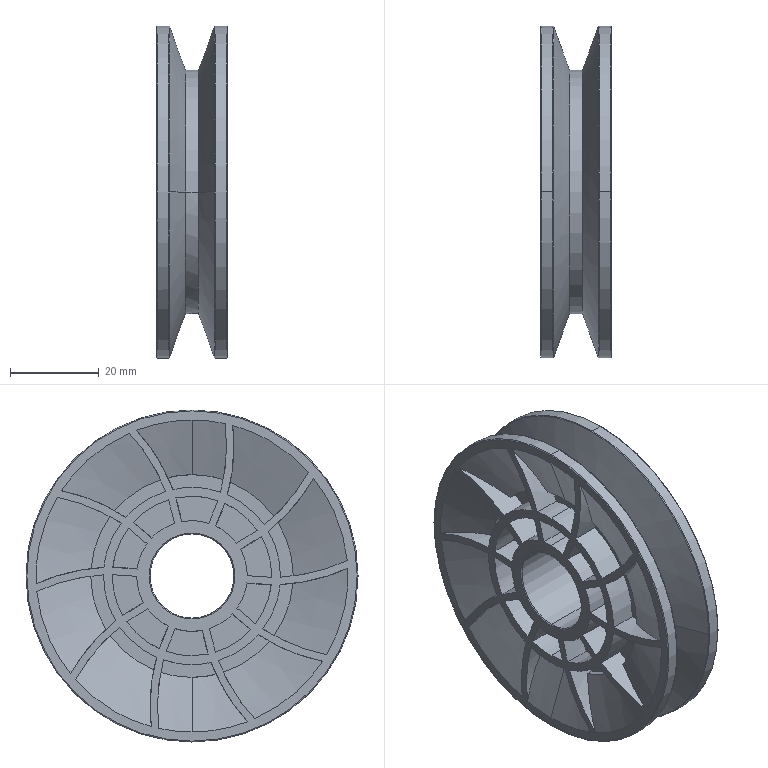Part | STEP file | V00-000000627 | 1 solid | 393 faces | box 16 x 75 x 75 mm | volume 34582 mm3 | cylinder 196 | plane 122 | cone 50 | spline 17 | torus 8 | commonest cylinder face diameters 80 x40 83.306 x40 25 x24 36 x24 40 x24 45.74 x24